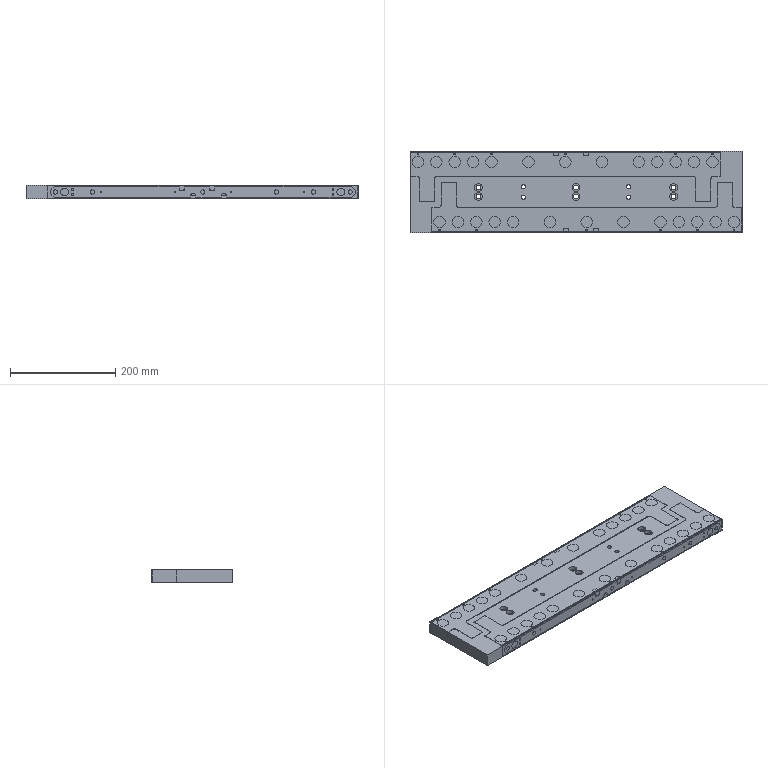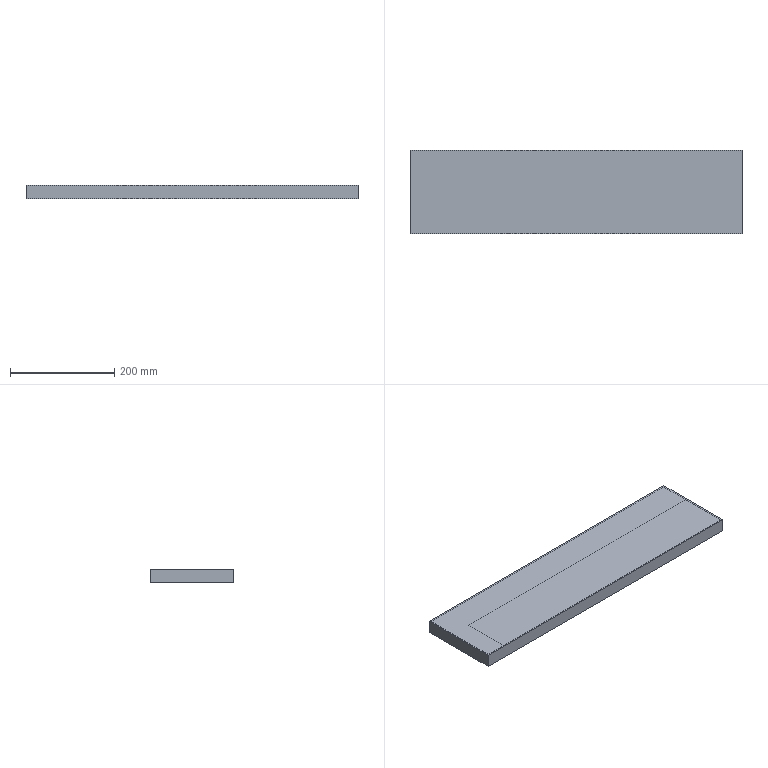CAM job | NX | 3+2 milling, drilling | part box 631 x 154 x 25 mm | stock box 637 x 160 x 26 mm
Tools:
number,name,description,diameter,corner_radius,flute_length,length,flutes
7,D6A45,Milling Tool-5 Parameters,6.0,0.0,3.0,3.0,2
9,10.5ZT,Drilling Tool,9.0,0.0,35.0,50.0,2
17,7.8ZT,Drilling Tool,7.8,0.0,35.0,50.0,2
18,8.0JD,Milling Tool-5 Parameters,8.0,0.0,30.0,30.0,4
10,D10,Milling Tool-5 Parameters,10.0,0.0,50.0,75.0,2
1,D63,Milling Tool-5 Parameters,63.0,0.0,50.0,75.0,2
13,3.3ZT,Drilling Tool,3.3,0.0,35.0,50.0,2
16,15.5ZT,Drilling Tool,16.0,0.0,35.0,50.0,2
8,D8JING,Milling Tool-5 Parameters,8.0,0.0,50.0,75.0,2
12,2.5ZT,Drilling Tool,2.5,0.0,35.0,50.0,2
15,5.5ZT,Drilling Tool,5.5,0.0,35.0,50.0,2
11,D10JING,Milling Tool-5 Parameters,10.0,0.0,50.0,75.0,2
16,8.5ZT,Drilling Tool,8.5,0.0,35.0,50.0,2
14,M4,Milling Tool-5 Parameters,3.3,0.0,30.0,30.0,4
19,M3,Milling Tool-5 Parameters,2.5,0.0,30.0,30.0,4
Operations:
program,operation,operation_type,tool,method,geometry_group,spindle_rpm,surface_speed,feed_per_tooth,feed_cut,feed_plunge,cut_length_mm,path_length_mm,cut_time_min,machine_time_min
1打工装孔,DRILLING,Operation,D6A45,METHOD,A,3000.0,56.0,0.0333,200.0,0.0,40.0,630.48,0.2,0.259
1打工装孔,DRILLING_COPY,Operation,10.5ZT,METHOD,A,2000.0,56.0,0.05,200.0,0.0,190.223,878.283,0.9511,1.02
1打工装孔,DRILLING_COPY_COPY,Operation,7.8ZT,METHOD,A,2000.0,56.0,0.05,200.0,0.0,127.373,564.217,0.6369,0.6806
1打工装孔,DRILLING_COPY_COPY_COPY,Operation,8.0JD,METHOD,A,1000.0,25.0,0.025,50.0,0.0,116.0,541.47,2.32,2.362
1打工装孔,HOLE_MILLING,CylinderMilling,D10,METHOD,A,7000.0,219.0,0.1429,2000.0,100.0,896.88,1714.88,0.4484,0.5302
2,FLOOR_WALL,VolumeBased25DMillingOperation,D63,METHOD,A,6500.0,1286.0,0.0962,1250.0,100.0,2946.797,3000.797,2.357,2.363
2,DRILLING_COPY_1,Operation,D6A45,METHOD,A,3000.0,56.0,0.0333,200.0,0.0,193.8,2010.68,0.969,1.151
2,DRILLING_COPY_2,Operation,3.3ZT,METHOD,A,2000.0,20.0,0.025,100.0,0.0,359.897,1962.503,3.599,3.759
2,DRILLING_COPY_2_COPY_2,Operation,M4,METHOD,A,200.0,2.0,0.175,140.0,0.0,336.0,1914.709,2.4,2.558
2,DRILLING_COPY_2_COPY,Operation,15.5ZT,METHOD,A,1000.0,50.0,0.1,200.0,0.0,865.979,3110.711,4.33,4.554
2,HOLE_MILLING_COPY,CylinderMilling,D10JING,METHOD,A,7000.0,219.0,0.1429,2000.0,100.0,8125.691,11056.84,4.063,4.356
2,ZLEVEL_PROFILE_COPY_3,ZLevelMilling,D10JING,METHOD,A,7000.0,219.0,0.1071,1500.0,1000.0,5572.308,9511.536,4.271,4.665
2,ZLEVEL_PROFILE_COPY_1_COPY_COPY_COPY_COPY_2,ZLevelMilling,D6A45,METHOD,A,7000.0,131.0,0.0714,1000.0,1000.0,1698.49,6087.189,1.698,2.137
3背面铣工装沉头-工装孔分中,HOLE_MILLING_COPY_1,CylinderMilling,D10,METHOD,B,7000.0,219.0,0.1429,2000.0,100.0,896.88,1716.435,0.4484,0.5304
4工装孔分中,FLOOR_WALL_COPY,VolumeBased25DMillingOperation,D63,METHOD,B,6500.0,1286.0,0.0962,1250.0,100.0,2946.797,3000.797,2.357,2.363
4工装孔分中,HOLE_MILLING_COPY_COPY,CylinderMilling,D10,METHOD,B,7000.0,219.0,0.1429,2000.0,100.0,8125.691,11056.84,4.063,4.356
4工装孔分中,ZLEVEL_PROFILE,ZLevelMilling,D8JING,METHOD,B,7000.0,175.0,0.2143,3000.0,1000.0,71282.668,71614.669,23.825,23.858
4工装孔分中,ZLEVEL_PROFILE_COPY_1_COPY_COPY_COPY_COPY_2_COPY,ZLevelMilling,D6A45,METHOD,B,7000.0,131.0,0.0714,1000.0,1000.0,1698.49,5397.665,1.698,2.068
4工装孔分中,ZLEVEL_PROFILE_COPY_1_COPY_COPY_COPY_COPY_2_COPY_COPY_1,ZLevelMilling,D6A45,METHOD,B,7000.0,131.0,0.0714,1000.0,1000.0,2926.232,3621.622,2.926,2.996
4工装孔分中,DRILLING_COPY_1_COPY_1,Operation,D6A45,METHOD,B,3000.0,56.0,0.0333,200.0,0.0,61.2,1365.109,0.306,0.4364
4工装孔分中,ZLEVEL_PROFILE_COPY,ZLevelMilling,D8JING,METHOD,B,7000.0,175.0,0.0714,1000.0,1000.0,15696.834,16135.572,15.697,15.741
5,DRILLING_COPY_1_COPY,Operation,D6A45,METHOD,C,3000.0,56.0,0.0333,200.0,0.0,61.2,797.668,0.306,0.3796
5,DRILLING_COPY_1_COPY_COPY,Operation,D6A45,METHOD,C,3000.0,56.0,0.0333,200.0,0.0,18.4,491.907,0.092,0.1394
5,DRILLING_COPY_2_COPY_1,Operation,3.3ZT,METHOD,C,2000.0,20.0,0.025,100.0,0.0,55.966,694.914,0.5597,0.6236
5,DRILLING_COPY_2_COPY_2_COPY,Operation,M4,METHOD,C,200.0,2.0,0.175,140.0,0.0,52.0,686.983,0.3714,0.4349
5,DRILLING_COPY_2_COPY_1_COPY,Operation,2.5ZT,METHOD,C,2000.0,20.0,0.025,100.0,0.0,55.004,565.115,0.55,0.6011
5,DRILLING_COPY_2_COPY_1_COPY_COPY_1,Operation,M3,METHOD,C,200.0,1.0,0.125,100.0,0.0,52.0,559.107,0.52,0.5707
5,DRILLING_COPY_2_COPY_1_COPY_COPY,Operation,5.5ZT,METHOD,C,2000.0,34.0,0.0625,250.0,0.0,216.609,594.925,0.8664,0.9043
5,DRILLING_COPY_COPY_1,Operation,10.5ZT,METHOD,C,1000.0,28.0,0.05,100.0,0.0,204.408,996.824,2.044,2.123
5,DRILLING_COPY_COPY_COPY_1,Operation,7.8ZT,METHOD,C,2000.0,56.0,0.05,200.0,0.0,119.491,874.228,0.5975,0.6729
5,DRILLING_COPY_COPY_COPY_COPY,Operation,8.0JD,METHOD,C,1000.0,25.0,0.025,50.0,0.0,99.431,834.108,1.989,2.062
5,HOLE_MILLING_COPY_1_COPY,CylinderMilling,D10,METHOD,C,7000.0,219.0,0.1071,1500.0,100.0,1175.684,1888.684,0.7838,0.8551
5,ZLEVEL_PROFILE_COPY_1,ZLevelMilling,D10,METHOD,C,7000.0,175.0,0.2143,3000.0,1000.0,2564.153,2623.103,0.8862,0.8921
5,HOLE_MILLING_COPY_1_COPY_COPY,CylinderMilling,D10JING,METHOD,C,7000.0,219.0,0.0714,1000.0,100.0,284.501,997.501,0.2845,0.3558
5,ZLEVEL_PROFILE_COPY_2,ZLevelMilling,D10JING,METHOD,C,7000.0,219.0,0.0857,1200.0,100.0,1243.619,1307.619,1.036,1.043
5,111,ZLevelMilling,D8JING,METHOD,C,7000.0,175.0,0.1286,1800.0,100.0,941.697,1384.955,0.5232,0.5675
5,ZLEVEL_PROFILE_COPY_1_COPY_COPY_COPY_COPY_2_COPY_COPY,ZLevelMilling,D6A45,METHOD,C,7000.0,131.0,0.0714,1000.0,1000.0,1468.459,3798.161,1.468,1.701
5,ZLEVEL_PROFILE_COPY_1_COPY_COPY_COPY_COPY_2_COPY_COPY_COPY,ZLevelMilling,D6A45,METHOD,C,7000.0,131.0,0.0714,1000.0,1000.0,1235.168,1515.4,1.235,1.263
6氧化后精加工,刀补11,CylinderMilling,D10JING,METHOD,D,7000.0,219.0,0.0714,1000.0,100.0,1389.021,2794.021,1.389,1.53
7工装底板,DRILLING_COPY_3,Operation,D6A45,METHOD,E,3000.0,56.0,0.0333,200.0,0.0,40.0,630.48,0.2,0.259
7工装底板,DRILLING_COPY_COPY_2,Operation,8.5ZT,METHOD,E,2000.0,56.0,0.05,200.0,0.0,123.322,744.48,0.6166,0.6787
7工装底板,DRILLING_COPY_COPY_COPY_2,Operation,7.8ZT,METHOD,E,2000.0,56.0,0.05,200.0,0.0,81.373,472.217,0.4069,0.446
7工装底板,DRILLING_COPY_COPY_COPY_COPY_1,Operation,8.0JD,METHOD,E,1000.0,25.0,0.025,50.0,0.0,72.0,454.467,1.44,1.478
7工装底板,ZLEVEL_PROFILE_COPY_1_COPY_COPY_COPY_COPY_2_COPY_COPY_COPY_1,ZLevelMilling,D6A45,METHOD,E,7000.0,131.0,0.0714,1000.0,1000.0,96.177,591.651,0.0962,0.1457
7工装底板,PLANAR_MILL,PlanarMilling,D6A45,METHOD,E,7000.0,131.0,0.0893,1250.0,100.0,170.19,950.155,0.1362,0.2141